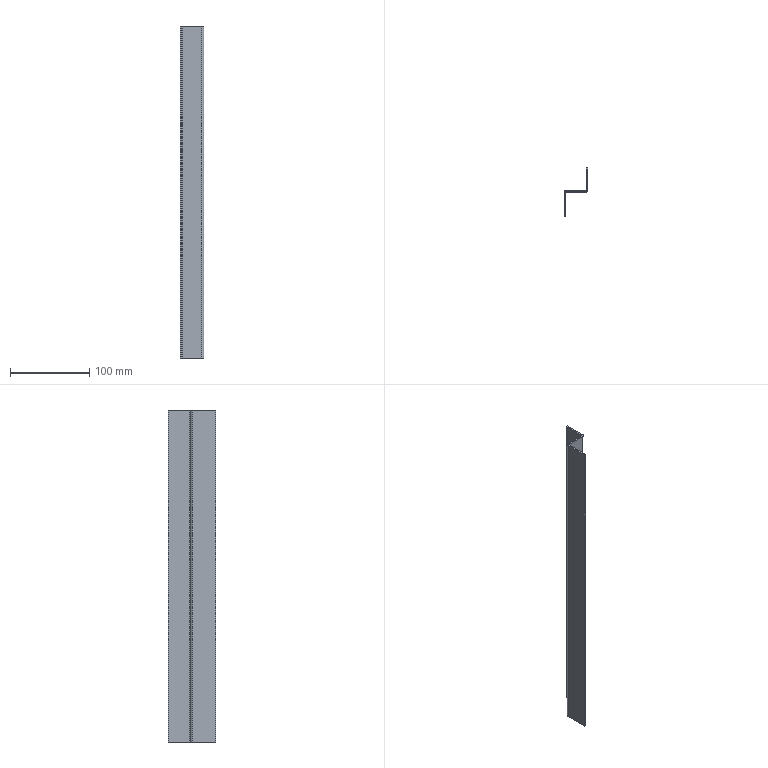Part | SolidWorks | features FlatPattern 1, SMBaseFlange 1, SheetMetal 1 | 1 solid | 22 faces | box 30 x 60 x 420 mm | volume 72668 mm3 | plane 18 | cylinder 4 | commonest cylinder face diameters 1.473 x2 5.473 x2
STEP:
#1=CARTESIAN_POINT('',(-0.3088,19.588,420.));
#2=VERTEX_POINT('',#1);
#3=CARTESIAN_POINT('',(-0.3088,21.588,420.));
#4=VERTEX_POINT('',#3);
#5=CARTESIAN_POINT('',(-0.3088,19.588,420.));
#6=DIRECTION('',(0.,1.,0.));
#7=VECTOR('',#6,1000.);
#8=LINE('',#5,#7);
#9=EDGE_CURVE('',#2,#4,#8,.T.);
#10=ORIENTED_EDGE('',*,*,#9,.F.);
#11=CARTESIAN_POINT('',(2.428,22.325,420.));
#12=VERTEX_POINT('',#11);
#13=CARTESIAN_POINT('',(-0.3088,22.325,420.));
#14=DIRECTION('',(0.,0.,-1.));
#15=DIRECTION('',(1.,0.,0.));
#16=AXIS2_PLACEMENT_3D('',#13,#14,#15);
#17=CIRCLE('',#16,2.737);
#18=EDGE_CURVE('',#12,#2,#17,.T.);
#19=ORIENTED_EDGE('',*,*,#18,.F.);
#20=CARTESIAN_POINT('',(0.4278,22.325,420.));
#21=VERTEX_POINT('',#20);
#22=CARTESIAN_POINT('',(0.4278,22.325,420.));
#23=DIRECTION('',(1.,0.,0.));
#24=VECTOR('',#23,1000.);
#25=LINE('',#22,#24);
#26=EDGE_CURVE('',#21,#12,#25,.T.);
#27=ORIENTED_EDGE('',*,*,#26,.F.);
#28=CARTESIAN_POINT('',(-0.3088,22.325,420.));
#29=DIRECTION('',(0.,0.,-1.));
#30=DIRECTION('',(1.,0.,0.));
#31=AXIS2_PLACEMENT_3D('',#28,#29,#30);
#32=CIRCLE('',#31,0.7366);
#33=EDGE_CURVE('',#21,#4,#32,.T.);
#34=ORIENTED_EDGE('',*,*,#33,.T.);
#35=EDGE_LOOP('',(#10,#19,#27,#34));
#36=FACE_OUTER_BOUND('',#35,.T.);
#37=CARTESIAN_POINT('',(-0.3088,19.588,420.));
#38=DIRECTION('',(0.,0.,1.));
#39=DIRECTION('',(1.,0.,0.));
#40=AXIS2_PLACEMENT_3D('',#37,#38,#39);
#41=PLANE('',#40);
#42=ADVANCED_FACE('',(#36),#41,.T.);
#43=CARTESIAN_POINT('',(-24.836,19.588,420.));
#44=VERTEX_POINT('',#43);
#45=CARTESIAN_POINT('',(2.428,19.588,420.));
#46=DIRECTION('',(-1.,0.,0.));
#47=VECTOR('',#46,1000.);
#48=LINE('',#45,#47);
#49=EDGE_CURVE('',#2,#44,#48,.T.);
#50=ORIENTED_EDGE('',*,*,#49,.F.);
#51=ORIENTED_EDGE('',*,*,#9,.T.);
#52=CARTESIAN_POINT('',(-24.836,21.588,420.));
#53=VERTEX_POINT('',#52);
#54=CARTESIAN_POINT('',(2.428,21.588,420.));
#55=DIRECTION('',(-1.,0.,0.));
#56=VECTOR('',#55,1000.);
#57=LINE('',#54,#56);
#58=EDGE_CURVE('',#4,#53,#57,.T.);
#59=ORIENTED_EDGE('',*,*,#58,.T.);
#60=CARTESIAN_POINT('',(-24.836,21.588,420.));
#61=DIRECTION('',(0.,-1.,0.));
#62=VECTOR('',#61,1000.);
#63=LINE('',#60,#62);
#64=EDGE_CURVE('',#53,#44,#63,.T.);
#65=ORIENTED_EDGE('',*,*,#64,.T.);
#66=EDGE_LOOP('',(#50,#51,#59,#65));
#67=FACE_OUTER_BOUND('',#66,.T.);
#68=CARTESIAN_POINT('',(0.4278,22.325,420.));
#69=DIRECTION('',(0.,0.,1.));
#70=DIRECTION('',(1.,0.,0.));
#71=AXIS2_PLACEMENT_3D('',#68,#69,#70);
#72=PLANE('',#71);
#73=ADVANCED_FACE('',(#67),#72,.T.);
#74=CARTESIAN_POINT('',(2.428,22.325,0.));
#75=VERTEX_POINT('',#74);
#76=CARTESIAN_POINT('',(0.4278,22.325,0.));
#77=VERTEX_POINT('',#76);
#78=CARTESIAN_POINT('',(2.428,22.325,0.));
#79=DIRECTION('',(-1.,0.,0.));
#80=VECTOR('',#79,1000.);
#81=LINE('',#78,#80);
#82=EDGE_CURVE('',#75,#77,#81,.T.);
#83=ORIENTED_EDGE('',*,*,#82,.F.);
#84=CARTESIAN_POINT('',(-0.3088,19.588,0.));
#85=VERTEX_POINT('',#84);
#86=CARTESIAN_POINT('',(-0.3088,22.325,0.));
#87=DIRECTION('',(0.,0.,-1.));
#88=DIRECTION('',(1.,0.,0.));
#89=AXIS2_PLACEMENT_3D('',#86,#87,#88);
#90=CIRCLE('',#89,2.737);
#91=EDGE_CURVE('',#75,#85,#90,.T.);
#92=ORIENTED_EDGE('',*,*,#91,.T.);
#93=CARTESIAN_POINT('',(-0.3088,21.588,0.));
#94=VERTEX_POINT('',#93);
#95=CARTESIAN_POINT('',(-0.3088,21.588,0.));
#96=DIRECTION('',(0.,-1.,0.));
#97=VECTOR('',#96,1000.);
#98=LINE('',#95,#97);
#99=EDGE_CURVE('',#94,#85,#98,.T.);
#100=ORIENTED_EDGE('',*,*,#99,.F.);
#101=CARTESIAN_POINT('',(-0.3088,22.325,0.));
#102=DIRECTION('',(0.,0.,-1.));
#103=DIRECTION('',(1.,0.,0.));
#104=AXIS2_PLACEMENT_3D('',#101,#102,#103);
#105=CIRCLE('',#104,0.7366);
#106=EDGE_CURVE('',#77,#94,#105,.T.);
#107=ORIENTED_EDGE('',*,*,#106,.F.);
#108=EDGE_LOOP('',(#83,#92,#100,#107));
#109=FACE_OUTER_BOUND('',#108,.T.);
#110=CARTESIAN_POINT('',(2.428,22.325,0.));
#111=DIRECTION('',(0.,0.,-1.));
#112=DIRECTION('',(-1.,0.,0.));
#113=AXIS2_PLACEMENT_3D('',#110,#111,#112);
#114=PLANE('',#113);
#115=ADVANCED_FACE('',(#109),#114,.T.);
#116=CARTESIAN_POINT('',(2.428,49.588,0.));
#117=VERTEX_POINT('',#116);
#118=CARTESIAN_POINT('',(2.428,49.588,0.));
#119=DIRECTION('',(0.,-1.,0.));
#120=VECTOR('',#119,1000.);
#121=LINE('',#118,#120);
#122=EDGE_CURVE('',#117,#75,#121,.T.);
#123=ORIENTED_EDGE('',*,*,#122,.T.);
#124=ORIENTED_EDGE('',*,*,#82,.T.);
#125=CARTESIAN_POINT('',(0.4278,49.588,0.));
#126=VERTEX_POINT('',#125);
#127=CARTESIAN_POINT('',(0.4278,49.588,0.));
#128=DIRECTION('',(0.,-1.,0.));
#129=VECTOR('',#128,1000.);
#130=LINE('',#127,#129);
#131=EDGE_CURVE('',#126,#77,#130,.T.);
#132=ORIENTED_EDGE('',*,*,#131,.F.);
#133=CARTESIAN_POINT('',(0.4278,49.588,0.));
#134=DIRECTION('',(1.,0.,0.));
#135=VECTOR('',#134,1000.);
#136=LINE('',#133,#135);
#137=EDGE_CURVE('',#126,#117,#136,.T.);
#138=ORIENTED_EDGE('',*,*,#137,.T.);
#139=EDGE_LOOP('',(#123,#124,#132,#138));
#140=FACE_OUTER_BOUND('',#139,.T.);
#141=CARTESIAN_POINT('',(-0.3088,21.588,0.));
#142=DIRECTION('',(0.,0.,-1.));
#143=DIRECTION('',(-1.,0.,0.));
#144=AXIS2_PLACEMENT_3D('',#141,#142,#143);
#145=PLANE('',#144);
#146=ADVANCED_FACE('',(#140),#145,.T.);
#147=CARTESIAN_POINT('',(-25.572,18.852,420.));
#148=VERTEX_POINT('',#147);
#149=CARTESIAN_POINT('',(-27.572,18.852,420.));
#150=VERTEX_POINT('',#149);
#151=CARTESIAN_POINT('',(-25.572,18.852,420.));
#152=DIRECTION('',(-1.,0.,0.));
#153=VECTOR('',#152,1000.);
#154=LINE('',#151,#153);
#155=EDGE_CURVE('',#148,#150,#154,.T.);
#156=ORIENTED_EDGE('',*,*,#155,.F.);
#157=CARTESIAN_POINT('',(-24.836,18.852,420.));
#158=DIRECTION('',(0.,0.,1.));
#159=DIRECTION('',(-1.,0.,0.));
#160=AXIS2_PLACEMENT_3D('',#157,#158,#159);
#161=CIRCLE('',#160,0.7366);
#162=EDGE_CURVE('',#44,#148,#161,.T.);
#163=ORIENTED_EDGE('',*,*,#162,.F.);
#164=ORIENTED_EDGE('',*,*,#64,.F.);
#165=CARTESIAN_POINT('',(-24.836,18.852,420.));
#166=DIRECTION('',(0.,0.,1.));
#167=DIRECTION('',(1.,0.,0.));
#168=AXIS2_PLACEMENT_3D('',#165,#166,#167);
#169=CIRCLE('',#168,2.737);
#170=EDGE_CURVE('',#53,#150,#169,.T.);
#171=ORIENTED_EDGE('',*,*,#170,.T.);
#172=EDGE_LOOP('',(#156,#163,#164,#171));
#173=FACE_OUTER_BOUND('',#172,.T.);
#174=CARTESIAN_POINT('',(-25.572,18.852,420.));
#175=DIRECTION('',(0.,0.,1.));
#176=DIRECTION('',(1.,0.,0.));
#177=AXIS2_PLACEMENT_3D('',#174,#175,#176);
#178=PLANE('',#177);
#179=ADVANCED_FACE('',(#173),#178,.T.);
#180=CARTESIAN_POINT('',(-25.572,-10.412,420.));
#181=VERTEX_POINT('',#180);
#182=CARTESIAN_POINT('',(-25.572,19.588,420.));
#183=DIRECTION('',(0.,-1.,0.));
#184=VECTOR('',#183,1000.);
#185=LINE('',#182,#184);
#186=EDGE_CURVE('',#148,#181,#185,.T.);
#187=ORIENTED_EDGE('',*,*,#186,.F.);
#188=ORIENTED_EDGE('',*,*,#155,.T.);
#189=CARTESIAN_POINT('',(-27.572,-10.412,420.));
#190=VERTEX_POINT('',#189);
#191=CARTESIAN_POINT('',(-27.572,19.588,420.));
#192=DIRECTION('',(0.,-1.,0.));
#193=VECTOR('',#192,1000.);
#194=LINE('',#191,#193);
#195=EDGE_CURVE('',#150,#190,#194,.T.);
#196=ORIENTED_EDGE('',*,*,#195,.T.);
#197=CARTESIAN_POINT('',(-25.572,-10.412,420.));
#198=DIRECTION('',(-1.,0.,0.));
#199=VECTOR('',#198,1000.);
#200=LINE('',#197,#199);
#201=EDGE_CURVE('',#181,#190,#200,.T.);
#202=ORIENTED_EDGE('',*,*,#201,.F.);
#203=EDGE_LOOP('',(#187,#188,#196,#202));
#204=FACE_OUTER_BOUND('',#203,.T.);
#205=CARTESIAN_POINT('',(-24.836,21.588,420.));
#206=DIRECTION('',(0.,0.,1.));
#207=DIRECTION('',(1.,0.,0.));
#208=AXIS2_PLACEMENT_3D('',#205,#206,#207);
#209=PLANE('',#208);
#210=ADVANCED_FACE('',(#204),#209,.T.);
#211=CARTESIAN_POINT('',(-24.836,19.588,0.));
#212=VERTEX_POINT('',#211);
#213=CARTESIAN_POINT('',(-24.836,21.588,0.));
#214=VERTEX_POINT('',#213);
#215=CARTESIAN_POINT('',(-24.836,19.588,0.));
#216=DIRECTION('',(0.,1.,0.));
#217=VECTOR('',#216,1000.);
#218=LINE('',#215,#217);
#219=EDGE_CURVE('',#212,#214,#218,.T.);
#220=ORIENTED_EDGE('',*,*,#219,.F.);
#221=CARTESIAN_POINT('',(-25.572,18.852,0.));
#222=VERTEX_POINT('',#221);
#223=CARTESIAN_POINT('',(-24.836,18.852,0.));
#224=DIRECTION('',(0.,0.,1.));
#225=DIRECTION('',(-1.,0.,0.));
#226=AXIS2_PLACEMENT_3D('',#223,#224,#225);
#227=CIRCLE('',#226,0.7366);
#228=EDGE_CURVE('',#212,#222,#227,.T.);
#229=ORIENTED_EDGE('',*,*,#228,.T.);
#230=CARTESIAN_POINT('',(-27.572,18.852,0.));
#231=VERTEX_POINT('',#230);
#232=CARTESIAN_POINT('',(-27.572,18.852,0.));
#233=DIRECTION('',(1.,0.,0.));
#234=VECTOR('',#233,1000.);
#235=LINE('',#232,#234);
#236=EDGE_CURVE('',#231,#222,#235,.T.);
#237=ORIENTED_EDGE('',*,*,#236,.F.);
#238=CARTESIAN_POINT('',(-24.836,18.852,0.));
#239=DIRECTION('',(0.,0.,1.));
#240=DIRECTION('',(1.,0.,0.));
#241=AXIS2_PLACEMENT_3D('',#238,#239,#240);
#242=CIRCLE('',#241,2.737);
#243=EDGE_CURVE('',#214,#231,#242,.T.);
#244=ORIENTED_EDGE('',*,*,#243,.F.);
#245=EDGE_LOOP('',(#220,#229,#237,#244));
#246=FACE_OUTER_BOUND('',#245,.T.);
#247=CARTESIAN_POINT('',(-24.836,19.588,0.));
#248=DIRECTION('',(0.,0.,-1.));
#249=DIRECTION('',(-1.,0.,0.));
#250=AXIS2_PLACEMENT_3D('',#247,#248,#249);
#251=PLANE('',#250);
#252=ADVANCED_FACE('',(#246),#251,.T.);
#253=CARTESIAN_POINT('',(2.428,19.588,0.));
#254=DIRECTION('',(-1.,0.,0.));
#255=VECTOR('',#254,1000.);
#256=LINE('',#253,#255);
#257=EDGE_CURVE('',#85,#212,#256,.T.);
#258=ORIENTED_EDGE('',*,*,#257,.T.);
#259=ORIENTED_EDGE('',*,*,#219,.T.);
#260=CARTESIAN_POINT('',(2.428,21.588,0.));
#261=DIRECTION('',(-1.,0.,0.));
#262=VECTOR('',#261,1000.);
#263=LINE('',#260,#262);
#264=EDGE_CURVE('',#94,#214,#263,.T.);
#265=ORIENTED_EDGE('',*,*,#264,.F.);
#266=ORIENTED_EDGE('',*,*,#99,.T.);
#267=EDGE_LOOP('',(#258,#259,#265,#266));
#268=FACE_OUTER_BOUND('',#267,.T.);
#269=CARTESIAN_POINT('',(-27.572,18.852,0.));
#270=DIRECTION('',(0.,0.,-1.));
#271=DIRECTION('',(-1.,0.,0.));
#272=AXIS2_PLACEMENT_3D('',#269,#270,#271);
#273=PLANE('',#272);
#274=ADVANCED_FACE('',(#268),#273,.T.);
#275=CARTESIAN_POINT('',(-27.572,-10.412,0.));
#276=VERTEX_POINT('',#275);
#277=CARTESIAN_POINT('',(-27.572,19.588,0.));
#278=DIRECTION('',(0.,-1.,0.));
#279=VECTOR('',#278,1000.);
#280=LINE('',#277,#279);
#281=EDGE_CURVE('',#231,#276,#280,.T.);
#282=ORIENTED_EDGE('',*,*,#281,.T.);
#283=CARTESIAN_POINT('',(-27.572,-10.412,420.));
#284=DIRECTION('',(0.,0.,-1.));
#285=VECTOR('',#284,1000.);
#286=LINE('',#283,#285);
#287=EDGE_CURVE('',#190,#276,#286,.T.);
#288=ORIENTED_EDGE('',*,*,#287,.F.);
#289=ORIENTED_EDGE('',*,*,#195,.F.);
#290=CARTESIAN_POINT('',(-27.572,18.852,420.));
#291=DIRECTION('',(0.,0.,-1.));
#292=VECTOR('',#291,1000.);
#293=LINE('',#290,#292);
#294=EDGE_CURVE('',#150,#231,#293,.T.);
#295=ORIENTED_EDGE('',*,*,#294,.T.);
#296=EDGE_LOOP('',(#282,#288,#289,#295));
#297=FACE_OUTER_BOUND('',#296,.T.);
#298=CARTESIAN_POINT('',(-27.572,19.588,420.));
#299=DIRECTION('',(1.,0.,0.));
#300=DIRECTION('',(0.,1.,0.));
#301=AXIS2_PLACEMENT_3D('',#298,#299,#300);
#302=PLANE('',#301);
#303=ADVANCED_FACE('',(#297),#302,.F.);
#304=CARTESIAN_POINT('',(-25.572,-10.412,0.));
#305=VERTEX_POINT('',#304);
#306=CARTESIAN_POINT('',(-25.572,-10.412,0.));
#307=DIRECTION('',(-1.,0.,0.));
#308=VECTOR('',#307,1000.);
#309=LINE('',#306,#308);
#310=EDGE_CURVE('',#305,#276,#309,.T.);
#311=ORIENTED_EDGE('',*,*,#310,.F.);
#312=CARTESIAN_POINT('',(-25.572,-10.412,420.));
#313=DIRECTION('',(0.,0.,-1.));
#314=VECTOR('',#313,1000.);
#315=LINE('',#312,#314);
#316=EDGE_CURVE('',#181,#305,#315,.T.);
#317=ORIENTED_EDGE('',*,*,#316,.F.);
#318=ORIENTED_EDGE('',*,*,#201,.T.);
#319=ORIENTED_EDGE('',*,*,#287,.T.);
#320=EDGE_LOOP('',(#311,#317,#318,#319));
#321=FACE_OUTER_BOUND('',#320,.T.);
#322=CARTESIAN_POINT('',(-25.572,-10.412,420.));
#323=DIRECTION('',(0.,-1.,0.));
#324=DIRECTION('',(0.,0.,-1.));
#325=AXIS2_PLACEMENT_3D('',#322,#323,#324);
#326=PLANE('',#325);
#327=ADVANCED_FACE('',(#321),#326,.T.);
#328=CARTESIAN_POINT('',(-25.572,19.588,0.));
#329=DIRECTION('',(0.,-1.,0.));
#330=VECTOR('',#329,1000.);
#331=LINE('',#328,#330);
#332=EDGE_CURVE('',#222,#305,#331,.T.);
#333=ORIENTED_EDGE('',*,*,#332,.F.);
#334=CARTESIAN_POINT('',(-25.572,18.852,420.));
#335=DIRECTION('',(0.,0.,-1.));
#336=VECTOR('',#335,1000.);
#337=LINE('',#334,#336);
#338=EDGE_CURVE('',#148,#222,#337,.T.);
#339=ORIENTED_EDGE('',*,*,#338,.F.);
#340=ORIENTED_EDGE('',*,*,#186,.T.);
#341=ORIENTED_EDGE('',*,*,#316,.T.);
#342=EDGE_LOOP('',(#333,#339,#340,#341));
#343=FACE_OUTER_BOUND('',#342,.T.);
#344=CARTESIAN_POINT('',(-25.572,19.588,420.));
#345=DIRECTION('',(1.,0.,0.));
#346=DIRECTION('',(0.,1.,0.));
#347=AXIS2_PLACEMENT_3D('',#344,#345,#346);
#348=PLANE('',#347);
#349=ADVANCED_FACE('',(#343),#348,.T.);
#350=ORIENTED_EDGE('',*,*,#228,.F.);
#351=CARTESIAN_POINT('',(-24.836,19.588,420.));
#352=DIRECTION('',(0.,0.,-1.));
#353=VECTOR('',#352,1000.);
#354=LINE('',#351,#353);
#355=EDGE_CURVE('',#44,#212,#354,.T.);
#356=ORIENTED_EDGE('',*,*,#355,.F.);
#357=ORIENTED_EDGE('',*,*,#162,.T.);
#358=ORIENTED_EDGE('',*,*,#338,.T.);
#359=EDGE_LOOP('',(#350,#356,#357,#358));
#360=FACE_OUTER_BOUND('',#359,.T.);
#361=CARTESIAN_POINT('',(-24.836,18.852,420.));
#362=DIRECTION('',(0.,0.,-1.));
#363=DIRECTION('',(-1.,0.,0.));
#364=AXIS2_PLACEMENT_3D('',#361,#362,#363);
#365=CYLINDRICAL_SURFACE('',#364,0.7366);
#366=ADVANCED_FACE('',(#360),#365,.F.);
#367=ORIENTED_EDGE('',*,*,#257,.F.);
#368=CARTESIAN_POINT('',(-0.3088,19.588,420.));
#369=DIRECTION('',(0.,0.,-1.));
#370=VECTOR('',#369,1000.);
#371=LINE('',#368,#370);
#372=EDGE_CURVE('',#2,#85,#371,.T.);
#373=ORIENTED_EDGE('',*,*,#372,.F.);
#374=ORIENTED_EDGE('',*,*,#49,.T.);
#375=ORIENTED_EDGE('',*,*,#355,.T.);
#376=EDGE_LOOP('',(#367,#373,#374,#375));
#377=FACE_OUTER_BOUND('',#376,.T.);
#378=CARTESIAN_POINT('',(2.428,19.588,420.));
#379=DIRECTION('',(0.,-1.,0.));
#380=DIRECTION('',(0.,0.,-1.));
#381=AXIS2_PLACEMENT_3D('',#378,#379,#380);
#382=PLANE('',#381);
#383=ADVANCED_FACE('',(#377),#382,.T.);
#384=ORIENTED_EDGE('',*,*,#91,.F.);
#385=CARTESIAN_POINT('',(2.428,22.325,420.));
#386=DIRECTION('',(0.,0.,-1.));
#387=VECTOR('',#386,1000.);
#388=LINE('',#385,#387);
#389=EDGE_CURVE('',#12,#75,#388,.T.);
#390=ORIENTED_EDGE('',*,*,#389,.F.);
#391=ORIENTED_EDGE('',*,*,#18,.T.);
#392=ORIENTED_EDGE('',*,*,#372,.T.);
#393=EDGE_LOOP('',(#384,#390,#391,#392));
#394=FACE_OUTER_BOUND('',#393,.T.);
#395=CARTESIAN_POINT('',(-0.3088,22.325,420.));
#396=DIRECTION('',(0.,0.,-1.));
#397=DIRECTION('',(-1.,0.,0.));
#398=AXIS2_PLACEMENT_3D('',#395,#396,#397);
#399=CYLINDRICAL_SURFACE('',#398,2.737);
#400=ADVANCED_FACE('',(#394),#399,.T.);
#401=ORIENTED_EDGE('',*,*,#122,.F.);
#402=CARTESIAN_POINT('',(2.428,49.588,420.));
#403=VERTEX_POINT('',#402);
#404=CARTESIAN_POINT('',(2.428,49.588,420.));
#405=DIRECTION('',(0.,0.,-1.));
#406=VECTOR('',#405,1000.);
#407=LINE('',#404,#406);
#408=EDGE_CURVE('',#403,#117,#407,.T.);
#409=ORIENTED_EDGE('',*,*,#408,.F.);
#410=CARTESIAN_POINT('',(2.428,49.588,420.));
#411=DIRECTION('',(0.,-1.,0.));
#412=VECTOR('',#411,1000.);
#413=LINE('',#410,#412);
#414=EDGE_CURVE('',#403,#12,#413,.T.);
#415=ORIENTED_EDGE('',*,*,#414,.T.);
#416=ORIENTED_EDGE('',*,*,#389,.T.);
#417=EDGE_LOOP('',(#401,#409,#415,#416));
#418=FACE_OUTER_BOUND('',#417,.T.);
#419=CARTESIAN_POINT('',(2.428,49.588,420.));
#420=DIRECTION('',(1.,0.,0.));
#421=DIRECTION('',(0.,1.,0.));
#422=AXIS2_PLACEMENT_3D('',#419,#420,#421);
#423=PLANE('',#422);
#424=ADVANCED_FACE('',(#418),#423,.T.);
#425=ORIENTED_EDGE('',*,*,#137,.F.);
#426=CARTESIAN_POINT('',(0.4278,49.588,420.));
#427=VERTEX_POINT('',#426);
#428=CARTESIAN_POINT('',(0.4278,49.588,420.));
#429=DIRECTION('',(0.,0.,-1.));
#430=VECTOR('',#429,1000.);
#431=LINE('',#428,#430);
#432=EDGE_CURVE('',#427,#126,#431,.T.);
#433=ORIENTED_EDGE('',*,*,#432,.F.);
#434=CARTESIAN_POINT('',(0.4278,49.588,420.));
#435=DIRECTION('',(1.,0.,0.));
#436=VECTOR('',#435,1000.);
#437=LINE('',#434,#436);
#438=EDGE_CURVE('',#427,#403,#437,.T.);
#439=ORIENTED_EDGE('',*,*,#438,.T.);
#440=ORIENTED_EDGE('',*,*,#408,.T.);
#441=EDGE_LOOP('',(#425,#433,#439,#440));
#442=FACE_OUTER_BOUND('',#441,.T.);
#443=CARTESIAN_POINT('',(0.4278,49.588,420.));
#444=DIRECTION('',(0.,1.,0.));
#445=DIRECTION('',(0.,0.,1.));
#446=AXIS2_PLACEMENT_3D('',#443,#444,#445);
#447=PLANE('',#446);
#448=ADVANCED_FACE('',(#442),#447,.T.);
#449=ORIENTED_EDGE('',*,*,#131,.T.);
#450=CARTESIAN_POINT('',(0.4278,22.325,420.));
#451=DIRECTION('',(0.,0.,-1.));
#452=VECTOR('',#451,1000.);
#453=LINE('',#450,#452);
#454=EDGE_CURVE('',#21,#77,#453,.T.);
#455=ORIENTED_EDGE('',*,*,#454,.F.);
#456=CARTESIAN_POINT('',(0.4278,49.588,420.));
#457=DIRECTION('',(0.,-1.,0.));
#458=VECTOR('',#457,1000.);
#459=LINE('',#456,#458);
#460=EDGE_CURVE('',#427,#21,#459,.T.);
#461=ORIENTED_EDGE('',*,*,#460,.F.);
#462=ORIENTED_EDGE('',*,*,#432,.T.);
#463=EDGE_LOOP('',(#449,#455,#461,#462));
#464=FACE_OUTER_BOUND('',#463,.T.);
#465=CARTESIAN_POINT('',(0.4278,49.588,420.));
#466=DIRECTION('',(1.,0.,0.));
#467=DIRECTION('',(0.,1.,0.));
#468=AXIS2_PLACEMENT_3D('',#465,#466,#467);
#469=PLANE('',#468);
#470=ADVANCED_FACE('',(#464),#469,.F.);
#471=ORIENTED_EDGE('',*,*,#106,.T.);
#472=CARTESIAN_POINT('',(-0.3088,21.588,420.));
#473=DIRECTION('',(0.,0.,-1.));
#474=VECTOR('',#473,1000.);
#475=LINE('',#472,#474);
#476=EDGE_CURVE('',#4,#94,#475,.T.);
#477=ORIENTED_EDGE('',*,*,#476,.F.);
#478=ORIENTED_EDGE('',*,*,#33,.F.);
#479=ORIENTED_EDGE('',*,*,#454,.T.);
#480=EDGE_LOOP('',(#471,#477,#478,#479));
#481=FACE_OUTER_BOUND('',#480,.T.);
#482=CARTESIAN_POINT('',(-0.3088,22.325,420.));
#483=DIRECTION('',(0.,0.,-1.));
#484=DIRECTION('',(-1.,0.,0.));
#485=AXIS2_PLACEMENT_3D('',#482,#483,#484);
#486=CYLINDRICAL_SURFACE('',#485,0.7366);
#487=ADVANCED_FACE('',(#481),#486,.F.);
#488=ORIENTED_EDGE('',*,*,#264,.T.);
#489=CARTESIAN_POINT('',(-24.836,21.588,420.));
#490=DIRECTION('',(0.,0.,-1.));
#491=VECTOR('',#490,1000.);
#492=LINE('',#489,#491);
#493=EDGE_CURVE('',#53,#214,#492,.T.);
#494=ORIENTED_EDGE('',*,*,#493,.F.);
#495=ORIENTED_EDGE('',*,*,#58,.F.);
#496=ORIENTED_EDGE('',*,*,#476,.T.);
#497=EDGE_LOOP('',(#488,#494,#495,#496));
#498=FACE_OUTER_BOUND('',#497,.T.);
#499=CARTESIAN_POINT('',(2.428,21.588,420.));
#500=DIRECTION('',(0.,-1.,0.));
#501=DIRECTION('',(0.,0.,-1.));
#502=AXIS2_PLACEMENT_3D('',#499,#500,#501);
#503=PLANE('',#502);
#504=ADVANCED_FACE('',(#498),#503,.F.);
#505=ORIENTED_EDGE('',*,*,#243,.T.);
#506=ORIENTED_EDGE('',*,*,#294,.F.);
#507=ORIENTED_EDGE('',*,*,#170,.F.);
#508=ORIENTED_EDGE('',*,*,#493,.T.);
#509=EDGE_LOOP('',(#505,#506,#507,#508));
#510=FACE_OUTER_BOUND('',#509,.T.);
#511=CARTESIAN_POINT('',(-24.836,18.852,420.));
#512=DIRECTION('',(0.,0.,-1.));
#513=DIRECTION('',(-1.,0.,0.));
#514=AXIS2_PLACEMENT_3D('',#511,#512,#513);
#515=CYLINDRICAL_SURFACE('',#514,2.737);
#516=ADVANCED_FACE('',(#510),#515,.T.);
#517=ORIENTED_EDGE('',*,*,#460,.T.);
#518=ORIENTED_EDGE('',*,*,#26,.T.);
#519=ORIENTED_EDGE('',*,*,#414,.F.);
#520=ORIENTED_EDGE('',*,*,#438,.F.);
#521=EDGE_LOOP('',(#517,#518,#519,#520));
#522=FACE_OUTER_BOUND('',#521,.T.);
#523=CARTESIAN_POINT('',(-24.836,18.852,420.));
#524=DIRECTION('',(0.,0.,-1.));
#525=DIRECTION('',(-1.,0.,0.));
#526=AXIS2_PLACEMENT_3D('',#523,#524,#525);
#527=PLANE('',#526);
#528=ADVANCED_FACE('',(#522),#527,.F.);
#529=ORIENTED_EDGE('',*,*,#281,.F.);
#530=ORIENTED_EDGE('',*,*,#236,.T.);
#531=ORIENTED_EDGE('',*,*,#332,.T.);
#532=ORIENTED_EDGE('',*,*,#310,.T.);
#533=EDGE_LOOP('',(#529,#530,#531,#532));
#534=FACE_OUTER_BOUND('',#533,.T.);
#535=CARTESIAN_POINT('',(-24.836,18.852,0.));
#536=DIRECTION('',(0.,0.,-1.));
#537=DIRECTION('',(-1.,0.,0.));
#538=AXIS2_PLACEMENT_3D('',#535,#536,#537);
#539=PLANE('',#538);
#540=ADVANCED_FACE('',(#534),#539,.T.);
#541=CLOSED_SHELL('',(#42,#73,#115,#146,#179,#210,#252,#274,#303,#327,#349,#366,#383,#400,#424,#448,#470,#487,#504,#516,#528,#540));
#542=MANIFOLD_SOLID_BREP('',#541);
#543=CARTESIAN_POINT('',(0.,0.,0.));
#544=DIRECTION('',(0.,0.,1.));
#545=DIRECTION('',(1.,0.,0.));
#546=AXIS2_PLACEMENT_3D('',#543,#544,#545);
#547=(LENGTH_UNIT()NAMED_UNIT(*)SI_UNIT(.MILLI.,.METRE.));
#548=UNCERTAINTY_MEASURE_WITH_UNIT(LENGTH_MEASURE(0.00001),#547,'','');
#549=(NAMED_UNIT(*)PLANE_ANGLE_UNIT()SI_UNIT($,.RADIAN.));
#550=(NAMED_UNIT(*)SI_UNIT($,.STERADIAN.)SOLID_ANGLE_UNIT());
#551=(GEOMETRIC_REPRESENTATION_CONTEXT(3)GLOBAL_UNCERTAINTY_ASSIGNED_CONTEXT((#548))GLOBAL_UNIT_ASSIGNED_CONTEXT((#547,#549,#550))REPRESENTATION_CONTEXT('',''));
#552=ADVANCED_BREP_SHAPE_REPRESENTATION('',(#542,#546),#551);